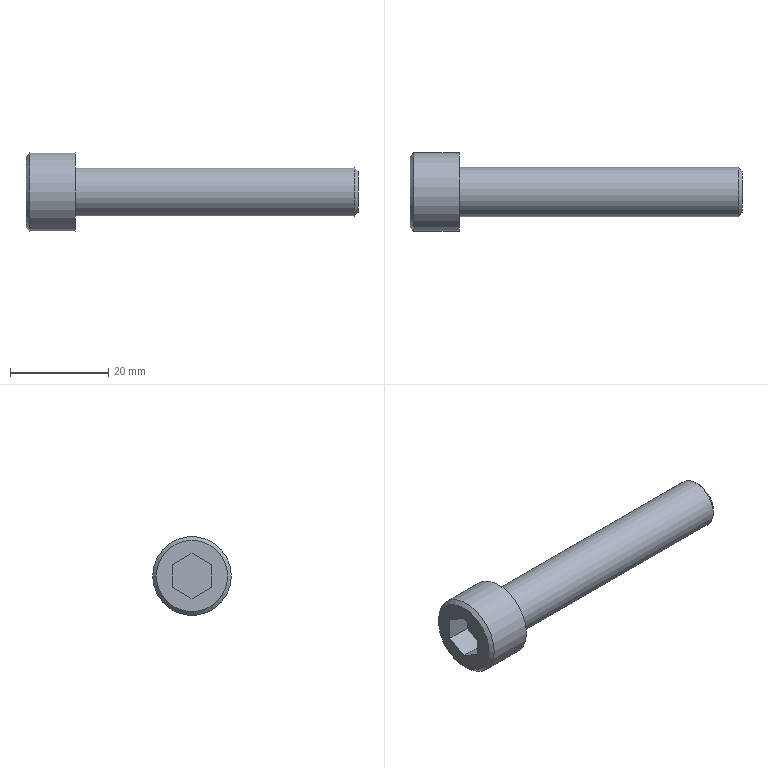Part | STEP file | solid 15 | 1 solid | 14 faces | box 67.5 x 16 x 16 mm | volume 6227 mm3 | plane 10 | cylinder 2 | cone 2 | commonest cylinder face diameters 10 x1 16 x1